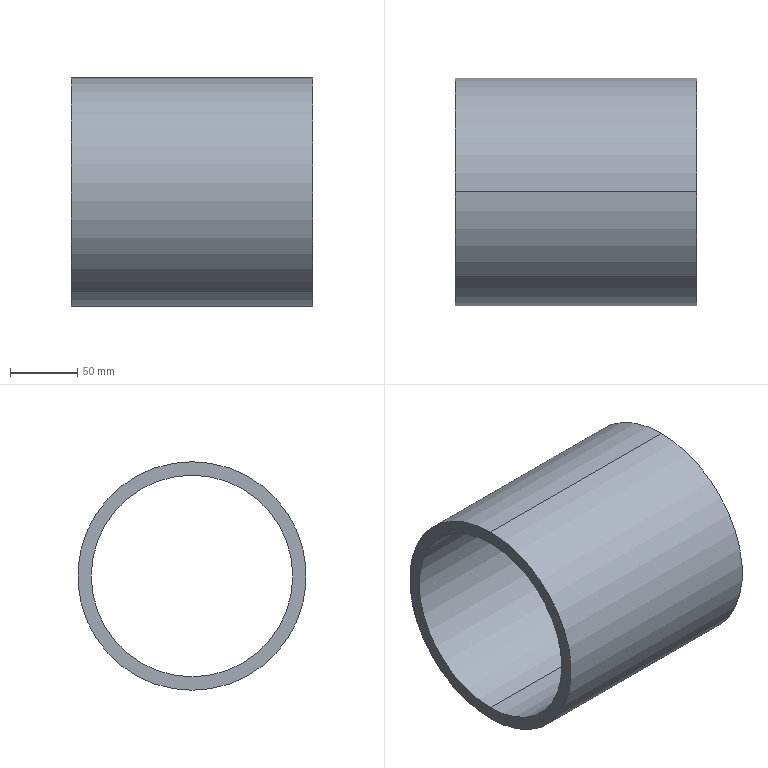Part | SolidWorks | features Extrusion 1 | 1 solid | 6 faces | box 180 x 170 x 170 mm | volume 904779 mm3 | cylinder 4 | plane 2 | commonest cylinder face diameters 150 x2 170 x2
STEP:
#1=CARTESIAN_POINT('',(180.,0.,75.));
#2=VERTEX_POINT('',#1);
#3=CARTESIAN_POINT('',(180.,0.,-75.));
#4=VERTEX_POINT('',#3);
#5=CARTESIAN_POINT('',(180.,0.,0.));
#6=DIRECTION('',(1.,0.,0.));
#7=DIRECTION('',(0.,0.,-1.));
#8=AXIS2_PLACEMENT_3D('',#5,#6,#7);
#9=CIRCLE('',#8,75.);
#10=EDGE_CURVE('',#2,#4,#9,.T.);
#11=ORIENTED_EDGE('',*,*,#10,.T.);
#12=CARTESIAN_POINT('',(0.,0.,-75.));
#13=VERTEX_POINT('',#12);
#14=CARTESIAN_POINT('',(180.,0.,-75.));
#15=DIRECTION('',(-1.,0.,0.));
#16=VECTOR('',#15,1000.);
#17=LINE('',#14,#16);
#18=EDGE_CURVE('',#4,#13,#17,.T.);
#19=ORIENTED_EDGE('',*,*,#18,.T.);
#20=CARTESIAN_POINT('',(0.,0.,75.));
#21=VERTEX_POINT('',#20);
#22=CARTESIAN_POINT('',(0.,0.,0.));
#23=DIRECTION('',(1.,0.,0.));
#24=DIRECTION('',(0.,0.,-1.));
#25=AXIS2_PLACEMENT_3D('',#22,#23,#24);
#26=CIRCLE('',#25,75.);
#27=EDGE_CURVE('',#21,#13,#26,.T.);
#28=ORIENTED_EDGE('',*,*,#27,.F.);
#29=CARTESIAN_POINT('',(180.,0.,75.));
#30=DIRECTION('',(-1.,0.,0.));
#31=VECTOR('',#30,1000.);
#32=LINE('',#29,#31);
#33=EDGE_CURVE('',#2,#21,#32,.T.);
#34=ORIENTED_EDGE('',*,*,#33,.F.);
#35=EDGE_LOOP('',(#11,#19,#28,#34));
#36=FACE_OUTER_BOUND('',#35,.T.);
#37=CARTESIAN_POINT('',(180.,0.,0.));
#38=DIRECTION('',(-1.,0.,0.));
#39=DIRECTION('',(0.,0.,1.));
#40=AXIS2_PLACEMENT_3D('',#37,#38,#39);
#41=CYLINDRICAL_SURFACE('',#40,75.);
#42=ADVANCED_FACE('',(#36),#41,.F.);
#43=CARTESIAN_POINT('',(180.,0.,-85.));
#44=VERTEX_POINT('',#43);
#45=CARTESIAN_POINT('',(180.,0.,85.));
#46=VERTEX_POINT('',#45);
#47=CARTESIAN_POINT('',(180.,0.,0.));
#48=DIRECTION('',(1.,0.,0.));
#49=DIRECTION('',(0.,0.,-1.));
#50=AXIS2_PLACEMENT_3D('',#47,#48,#49);
#51=CIRCLE('',#50,85.);
#52=EDGE_CURVE('',#44,#46,#51,.T.);
#53=ORIENTED_EDGE('',*,*,#52,.F.);
#54=CARTESIAN_POINT('',(0.,0.,-85.));
#55=VERTEX_POINT('',#54);
#56=CARTESIAN_POINT('',(180.,0.,-85.));
#57=DIRECTION('',(-1.,0.,0.));
#58=VECTOR('',#57,1000.);
#59=LINE('',#56,#58);
#60=EDGE_CURVE('',#44,#55,#59,.T.);
#61=ORIENTED_EDGE('',*,*,#60,.T.);
#62=CARTESIAN_POINT('',(0.,0.,85.));
#63=VERTEX_POINT('',#62);
#64=CARTESIAN_POINT('',(0.,0.,0.));
#65=DIRECTION('',(1.,0.,0.));
#66=DIRECTION('',(0.,0.,-1.));
#67=AXIS2_PLACEMENT_3D('',#64,#65,#66);
#68=CIRCLE('',#67,85.);
#69=EDGE_CURVE('',#55,#63,#68,.T.);
#70=ORIENTED_EDGE('',*,*,#69,.T.);
#71=CARTESIAN_POINT('',(180.,0.,85.));
#72=DIRECTION('',(-1.,0.,0.));
#73=VECTOR('',#72,1000.);
#74=LINE('',#71,#73);
#75=EDGE_CURVE('',#46,#63,#74,.T.);
#76=ORIENTED_EDGE('',*,*,#75,.F.);
#77=EDGE_LOOP('',(#53,#61,#70,#76));
#78=FACE_OUTER_BOUND('',#77,.T.);
#79=CARTESIAN_POINT('',(180.,0.,0.));
#80=DIRECTION('',(-1.,0.,0.));
#81=DIRECTION('',(0.,0.,1.));
#82=AXIS2_PLACEMENT_3D('',#79,#80,#81);
#83=CYLINDRICAL_SURFACE('',#82,85.);
#84=ADVANCED_FACE('',(#78),#83,.T.);
#85=CARTESIAN_POINT('',(180.,0.,0.));
#86=DIRECTION('',(1.,0.,0.));
#87=DIRECTION('',(0.,0.,-1.));
#88=AXIS2_PLACEMENT_3D('',#85,#86,#87);
#89=CIRCLE('',#88,85.);
#90=EDGE_CURVE('',#46,#44,#89,.T.);
#91=ORIENTED_EDGE('',*,*,#90,.T.);
#92=ORIENTED_EDGE('',*,*,#52,.T.);
#93=EDGE_LOOP('',(#91,#92));
#94=FACE_OUTER_BOUND('',#93,.T.);
#95=ORIENTED_EDGE('',*,*,#10,.F.);
#96=CARTESIAN_POINT('',(180.,0.,0.));
#97=DIRECTION('',(1.,0.,0.));
#98=DIRECTION('',(0.,0.,-1.));
#99=AXIS2_PLACEMENT_3D('',#96,#97,#98);
#100=CIRCLE('',#99,75.);
#101=EDGE_CURVE('',#4,#2,#100,.T.);
#102=ORIENTED_EDGE('',*,*,#101,.F.);
#103=EDGE_LOOP('',(#95,#102));
#104=FACE_BOUND('',#103,.T.);
#105=CARTESIAN_POINT('',(180.,0.,0.));
#106=DIRECTION('',(1.,0.,0.));
#107=DIRECTION('',(0.,0.,-1.));
#108=AXIS2_PLACEMENT_3D('',#105,#106,#107);
#109=PLANE('',#108);
#110=ADVANCED_FACE('',(#94,#104),#109,.T.);
#111=CARTESIAN_POINT('',(0.,0.,0.));
#112=DIRECTION('',(1.,0.,0.));
#113=DIRECTION('',(0.,0.,-1.));
#114=AXIS2_PLACEMENT_3D('',#111,#112,#113);
#115=CIRCLE('',#114,85.);
#116=EDGE_CURVE('',#63,#55,#115,.T.);
#117=ORIENTED_EDGE('',*,*,#116,.F.);
#118=ORIENTED_EDGE('',*,*,#69,.F.);
#119=EDGE_LOOP('',(#117,#118));
#120=FACE_OUTER_BOUND('',#119,.T.);
#121=ORIENTED_EDGE('',*,*,#27,.T.);
#122=CARTESIAN_POINT('',(0.,0.,0.));
#123=DIRECTION('',(1.,0.,0.));
#124=DIRECTION('',(0.,0.,-1.));
#125=AXIS2_PLACEMENT_3D('',#122,#123,#124);
#126=CIRCLE('',#125,75.);
#127=EDGE_CURVE('',#13,#21,#126,.T.);
#128=ORIENTED_EDGE('',*,*,#127,.T.);
#129=EDGE_LOOP('',(#121,#128));
#130=FACE_BOUND('',#129,.T.);
#131=CARTESIAN_POINT('',(0.,0.,0.));
#132=DIRECTION('',(1.,0.,0.));
#133=DIRECTION('',(0.,0.,-1.));
#134=AXIS2_PLACEMENT_3D('',#131,#132,#133);
#135=PLANE('',#134);
#136=ADVANCED_FACE('',(#120,#130),#135,.F.);
#137=ORIENTED_EDGE('',*,*,#60,.F.);
#138=ORIENTED_EDGE('',*,*,#90,.F.);
#139=ORIENTED_EDGE('',*,*,#75,.T.);
#140=ORIENTED_EDGE('',*,*,#116,.T.);
#141=EDGE_LOOP('',(#137,#138,#139,#140));
#142=FACE_OUTER_BOUND('',#141,.T.);
#143=CARTESIAN_POINT('',(180.,0.,0.));
#144=DIRECTION('',(-1.,0.,0.));
#145=DIRECTION('',(0.,0.,1.));
#146=AXIS2_PLACEMENT_3D('',#143,#144,#145);
#147=CYLINDRICAL_SURFACE('',#146,85.);
#148=ADVANCED_FACE('',(#142),#147,.T.);
#149=ORIENTED_EDGE('',*,*,#18,.F.);
#150=ORIENTED_EDGE('',*,*,#101,.T.);
#151=ORIENTED_EDGE('',*,*,#33,.T.);
#152=ORIENTED_EDGE('',*,*,#127,.F.);
#153=EDGE_LOOP('',(#149,#150,#151,#152));
#154=FACE_OUTER_BOUND('',#153,.T.);
#155=CARTESIAN_POINT('',(180.,0.,0.));
#156=DIRECTION('',(-1.,0.,0.));
#157=DIRECTION('',(0.,0.,1.));
#158=AXIS2_PLACEMENT_3D('',#155,#156,#157);
#159=CYLINDRICAL_SURFACE('',#158,75.);
#160=ADVANCED_FACE('',(#154),#159,.F.);
#161=CLOSED_SHELL('',(#42,#84,#110,#136,#148,#160));
#162=MANIFOLD_SOLID_BREP('',#161);
#163=CARTESIAN_POINT('',(0.,0.,0.));
#164=DIRECTION('',(0.,0.,1.));
#165=DIRECTION('',(1.,0.,0.));
#166=AXIS2_PLACEMENT_3D('',#163,#164,#165);
#167=(LENGTH_UNIT()NAMED_UNIT(*)SI_UNIT(.MILLI.,.METRE.));
#168=UNCERTAINTY_MEASURE_WITH_UNIT(LENGTH_MEASURE(0.00001),#167,'','');
#169=(NAMED_UNIT(*)PLANE_ANGLE_UNIT()SI_UNIT($,.RADIAN.));
#170=(NAMED_UNIT(*)SI_UNIT($,.STERADIAN.)SOLID_ANGLE_UNIT());
#171=(GEOMETRIC_REPRESENTATION_CONTEXT(3)GLOBAL_UNCERTAINTY_ASSIGNED_CONTEXT((#168))GLOBAL_UNIT_ASSIGNED_CONTEXT((#167,#169,#170))REPRESENTATION_CONTEXT('',''));
#172=ADVANCED_BREP_SHAPE_REPRESENTATION('',(#162,#166),#171);